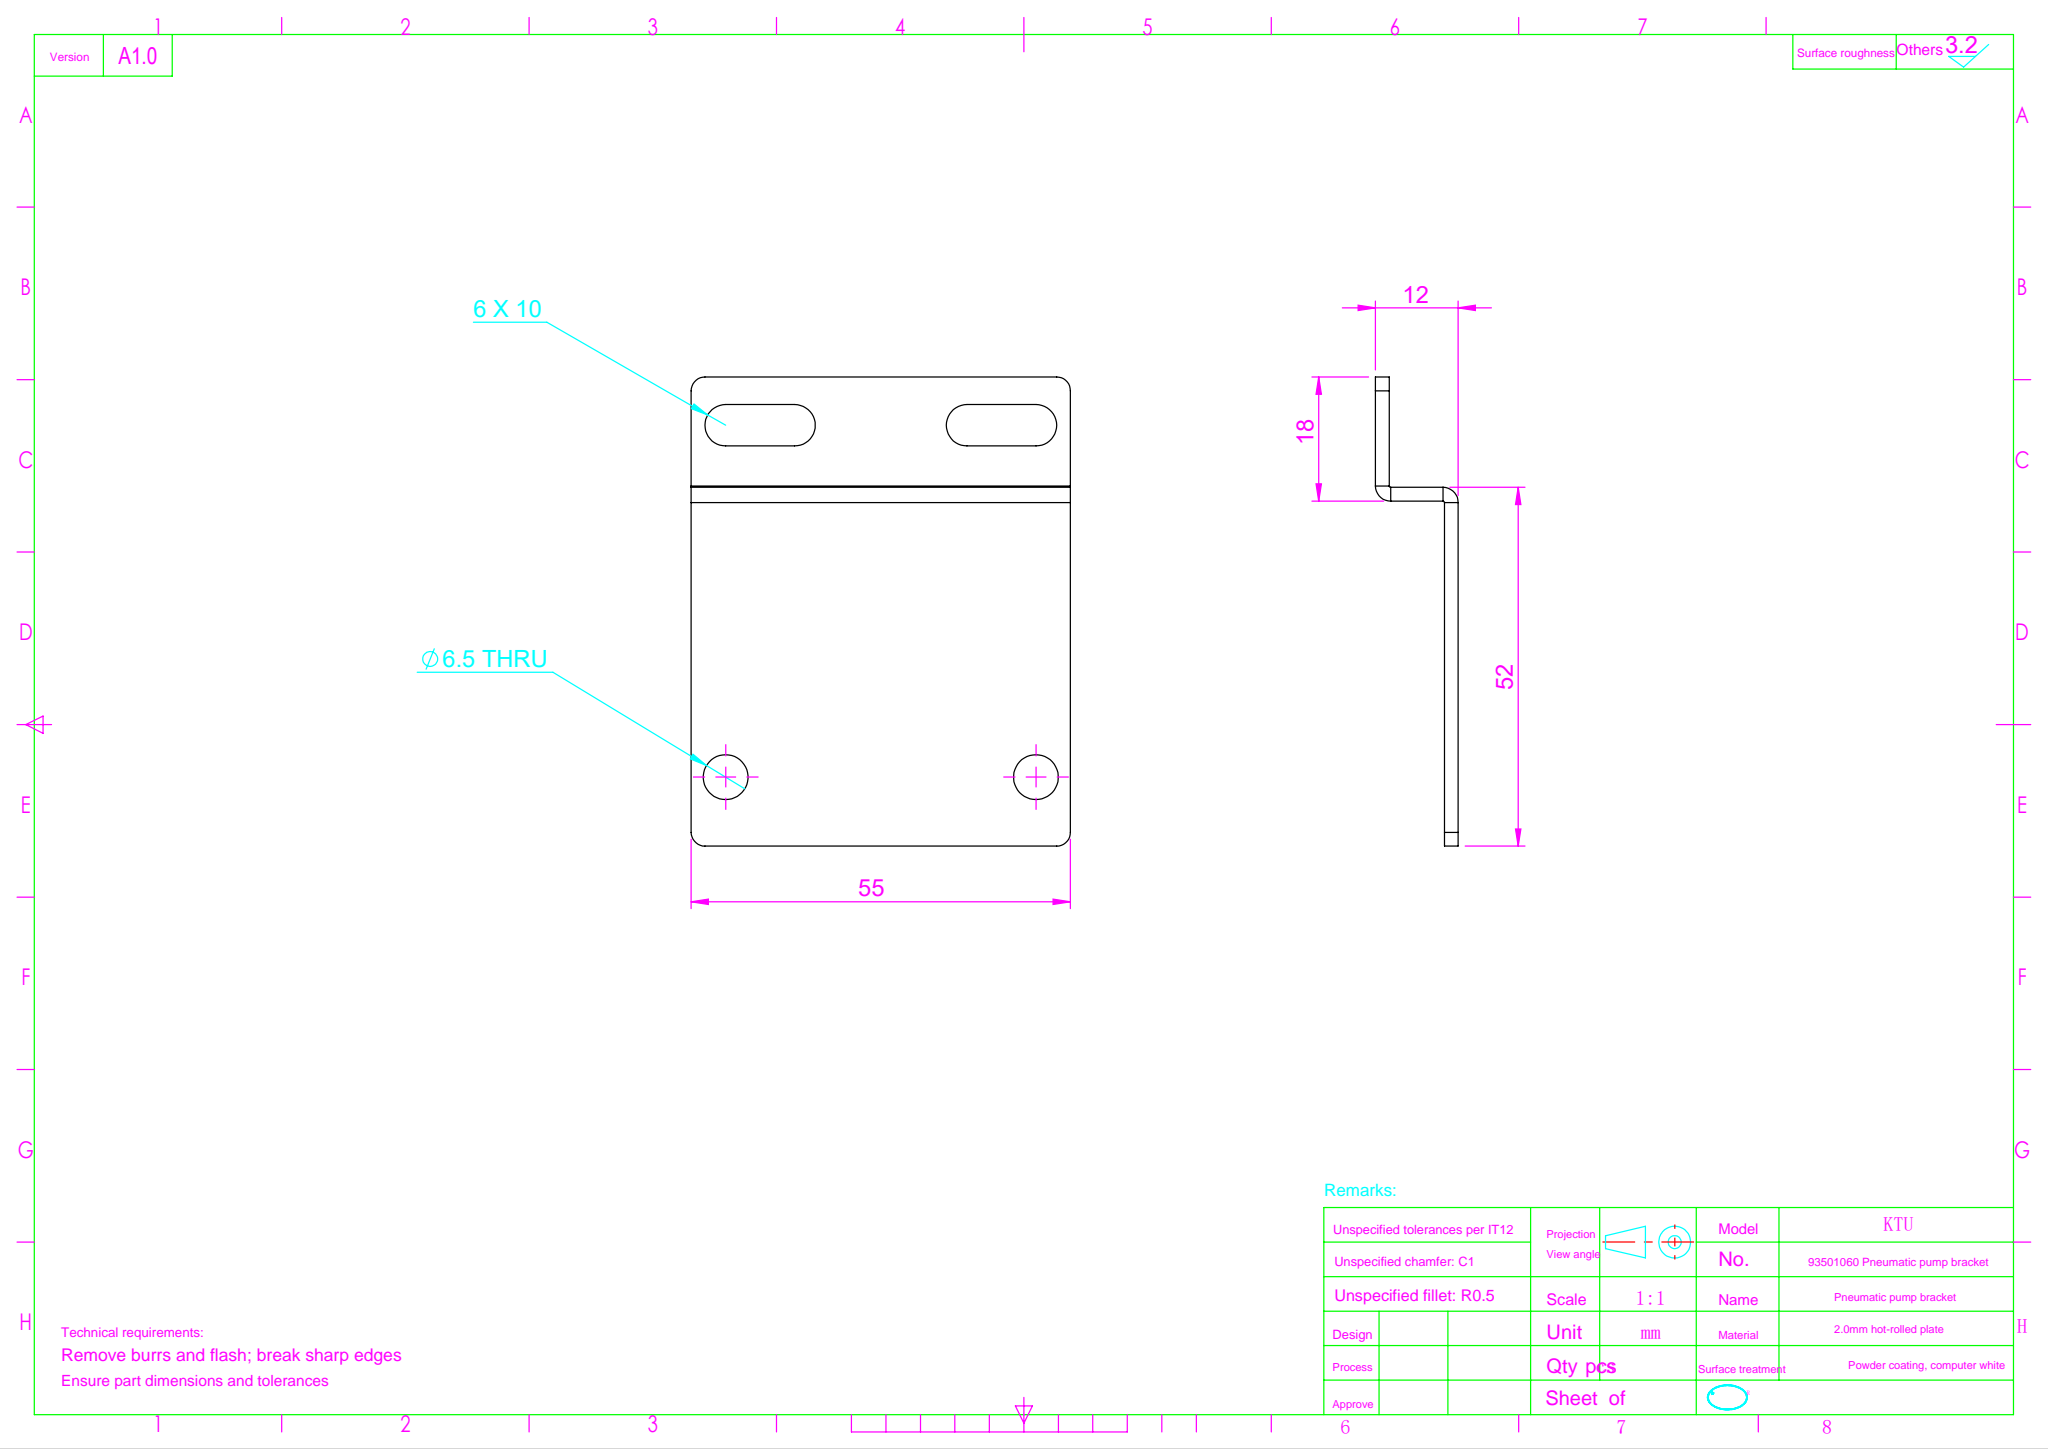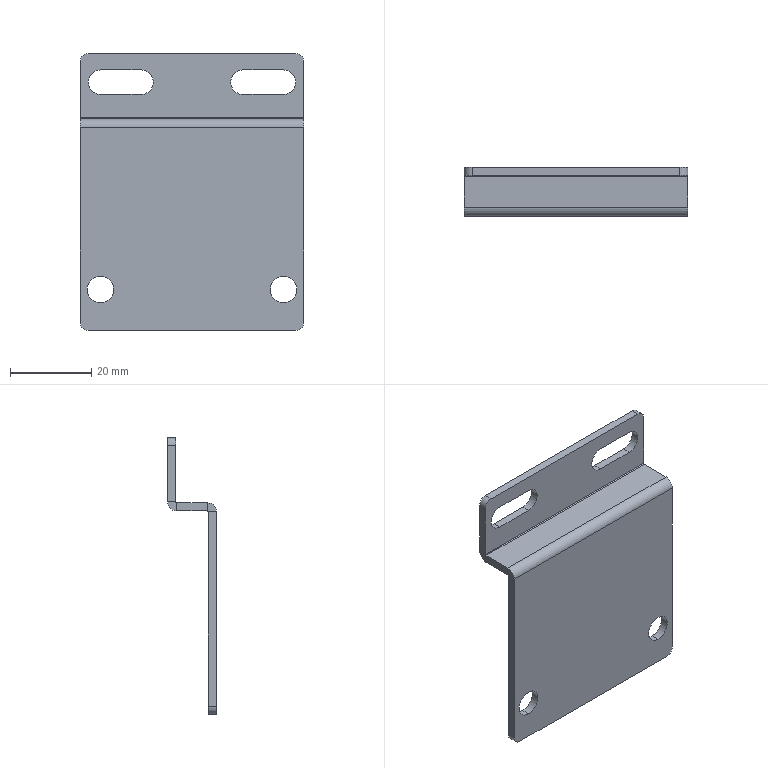Part | SolidWorks | features ICE 3, Fillet 1, FlatPattern 1, SMBaseFlange 1, SheetMetal 1 | 1 solid | 38 faces | box 55 x 12 x 68 mm | volume 7974 mm3 | plane 22 | cylinder 16 | commonest cylinder face diameters 4 x4 6 x4 6.5 x4 0.4 x2 4.4 x2